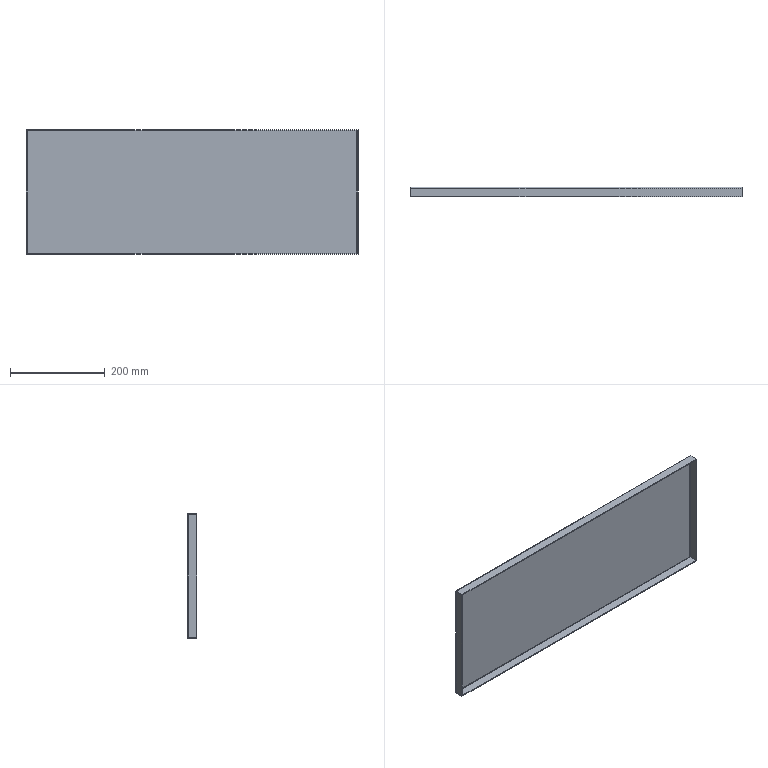Part | STEP file | Transformer Cover 1 | 1 solid | 34 faces | box 700 x 20 x 263 mm | volume 434709 mm3 | plane 26 | cylinder 8 | commonest cylinder face diameters 1 x4 5 x4
STEP:
#1=CARTESIAN_POINT('',(697.5,13.794,89.529));
#2=VERTEX_POINT('',#1);
#3=CARTESIAN_POINT('',(2.5,13.794,89.529));
#4=VERTEX_POINT('',#3);
#5=CARTESIAN_POINT('',(700.,13.794,89.529));
#6=DIRECTION('',(-1.,0.,0.));
#7=VECTOR('',#6,1000.);
#8=LINE('',#5,#7);
#9=EDGE_CURVE('',#2,#4,#8,.T.);
#10=ORIENTED_EDGE('',*,*,#9,.F.);
#11=CARTESIAN_POINT('',(697.5,13.794,-168.471));
#12=VERTEX_POINT('',#11);
#13=CARTESIAN_POINT('',(697.5,13.794,-170.971));
#14=DIRECTION('',(0.,0.,1.));
#15=VECTOR('',#14,1000.);
#16=LINE('',#13,#15);
#17=EDGE_CURVE('',#12,#2,#16,.T.);
#18=ORIENTED_EDGE('',*,*,#17,.F.);
#19=CARTESIAN_POINT('',(2.5,13.794,-168.471));
#20=VERTEX_POINT('',#19);
#21=CARTESIAN_POINT('',(700.,13.794,-168.471));
#22=DIRECTION('',(1.,0.,0.));
#23=VECTOR('',#22,1000.);
#24=LINE('',#21,#23);
#25=EDGE_CURVE('',#20,#12,#24,.T.);
#26=ORIENTED_EDGE('',*,*,#25,.F.);
#27=CARTESIAN_POINT('',(2.5,13.794,-170.971));
#28=DIRECTION('',(0.,0.,-1.));
#29=VECTOR('',#28,1000.);
#30=LINE('',#27,#29);
#31=EDGE_CURVE('',#4,#20,#30,.T.);
#32=ORIENTED_EDGE('',*,*,#31,.F.);
#33=EDGE_LOOP('',(#10,#18,#26,#32));
#34=FACE_OUTER_BOUND('',#33,.T.);
#35=CARTESIAN_POINT('',(700.,13.794,-170.971));
#36=DIRECTION('',(0.,-1.,0.));
#37=DIRECTION('',(0.,0.,-1.));
#38=AXIS2_PLACEMENT_3D('',#35,#36,#37);
#39=PLANE('',#38);
#40=ADVANCED_FACE('',(#34),#39,.F.);
#41=CARTESIAN_POINT('',(0.05051,11.794,89.529));
#42=VERTEX_POINT('',#41);
#43=CARTESIAN_POINT('',(0.,11.294,89.529));
#44=VERTEX_POINT('',#43);
#45=CARTESIAN_POINT('',(2.5,11.294,89.529));
#46=DIRECTION('',(0.,0.,1.));
#47=DIRECTION('',(-1.,0.,0.));
#48=AXIS2_PLACEMENT_3D('',#45,#46,#47);
#49=CIRCLE('',#48,2.5);
#50=EDGE_CURVE('',#42,#44,#49,.T.);
#51=ORIENTED_EDGE('',*,*,#50,.F.);
#52=CARTESIAN_POINT('',(2.5,11.294,89.529));
#53=DIRECTION('',(0.,0.,-1.));
#54=DIRECTION('',(-1.,0.,0.));
#55=AXIS2_PLACEMENT_3D('',#52,#53,#54);
#56=CIRCLE('',#55,2.5);
#57=EDGE_CURVE('',#42,#4,#56,.T.);
#58=ORIENTED_EDGE('',*,*,#57,.T.);
#59=ORIENTED_EDGE('',*,*,#31,.T.);
#60=CARTESIAN_POINT('',(0.05051,11.794,-168.471));
#61=VERTEX_POINT('',#60);
#62=CARTESIAN_POINT('',(2.5,11.294,-168.471));
#63=DIRECTION('',(0.,0.,1.));
#64=DIRECTION('',(-1.,0.,0.));
#65=AXIS2_PLACEMENT_3D('',#62,#63,#64);
#66=CIRCLE('',#65,2.5);
#67=EDGE_CURVE('',#20,#61,#66,.T.);
#68=ORIENTED_EDGE('',*,*,#67,.T.);
#69=CARTESIAN_POINT('',(0.,11.294,-168.471));
#70=VERTEX_POINT('',#69);
#71=CARTESIAN_POINT('',(2.5,11.294,-168.471));
#72=DIRECTION('',(0.,0.,1.));
#73=DIRECTION('',(-1.,0.,0.));
#74=AXIS2_PLACEMENT_3D('',#71,#72,#73);
#75=CIRCLE('',#74,2.5);
#76=EDGE_CURVE('',#61,#70,#75,.T.);
#77=ORIENTED_EDGE('',*,*,#76,.T.);
#78=CARTESIAN_POINT('',(0.,11.294,-168.471));
#79=DIRECTION('',(0.,0.,1.));
#80=VECTOR('',#79,1000.);
#81=LINE('',#78,#80);
#82=EDGE_CURVE('',#70,#44,#81,.T.);
#83=ORIENTED_EDGE('',*,*,#82,.T.);
#84=EDGE_LOOP('',(#51,#58,#59,#68,#77,#83));
#85=FACE_OUTER_BOUND('',#84,.T.);
#86=CARTESIAN_POINT('',(2.5,11.294,-168.471));
#87=DIRECTION('',(0.,0.,-1.));
#88=DIRECTION('',(-1.,0.,0.));
#89=AXIS2_PLACEMENT_3D('',#86,#87,#88);
#90=CYLINDRICAL_SURFACE('',#89,2.5);
#91=ADVANCED_FACE('',(#85),#90,.T.);
#92=ORIENTED_EDGE('',*,*,#9,.T.);
#93=CARTESIAN_POINT('',(0.,13.794,89.529));
#94=VERTEX_POINT('',#93);
#95=CARTESIAN_POINT('',(700.,13.794,89.529));
#96=DIRECTION('',(-1.,0.,0.));
#97=VECTOR('',#96,1000.);
#98=LINE('',#95,#97);
#99=EDGE_CURVE('',#4,#94,#98,.T.);
#100=ORIENTED_EDGE('',*,*,#99,.T.);
#101=CARTESIAN_POINT('',(0.,11.294,92.029));
#102=VERTEX_POINT('',#101);
#103=CARTESIAN_POINT('',(0.,11.294,89.529));
#104=DIRECTION('',(1.,0.,0.));
#105=DIRECTION('',(0.,0.,1.));
#106=AXIS2_PLACEMENT_3D('',#103,#104,#105);
#107=CIRCLE('',#106,2.5);
#108=EDGE_CURVE('',#94,#102,#107,.T.);
#109=ORIENTED_EDGE('',*,*,#108,.T.);
#110=CARTESIAN_POINT('',(700.,11.294,92.029));
#111=VERTEX_POINT('',#110);
#112=CARTESIAN_POINT('',(700.,11.294,92.029));
#113=DIRECTION('',(1.,0.,0.));
#114=VECTOR('',#113,1000.);
#115=LINE('',#112,#114);
#116=EDGE_CURVE('',#102,#111,#115,.T.);
#117=ORIENTED_EDGE('',*,*,#116,.T.);
#118=CARTESIAN_POINT('',(700.,13.794,89.529));
#119=VERTEX_POINT('',#118);
#120=CARTESIAN_POINT('',(700.,11.294,89.529));
#121=DIRECTION('',(-1.,0.,0.));
#122=DIRECTION('',(0.,0.,1.));
#123=AXIS2_PLACEMENT_3D('',#120,#121,#122);
#124=CIRCLE('',#123,2.5);
#125=EDGE_CURVE('',#111,#119,#124,.T.);
#126=ORIENTED_EDGE('',*,*,#125,.T.);
#127=CARTESIAN_POINT('',(700.,13.794,89.529));
#128=DIRECTION('',(-1.,0.,0.));
#129=VECTOR('',#128,1000.);
#130=LINE('',#127,#129);
#131=EDGE_CURVE('',#119,#2,#130,.T.);
#132=ORIENTED_EDGE('',*,*,#131,.T.);
#133=EDGE_LOOP('',(#92,#100,#109,#117,#126,#132));
#134=FACE_OUTER_BOUND('',#133,.T.);
#135=CARTESIAN_POINT('',(700.,11.294,89.529));
#136=DIRECTION('',(-1.,0.,0.));
#137=DIRECTION('',(0.,0.,1.));
#138=AXIS2_PLACEMENT_3D('',#135,#136,#137);
#139=CYLINDRICAL_SURFACE('',#138,2.5);
#140=ADVANCED_FACE('',(#134),#139,.T.);
#141=CARTESIAN_POINT('',(699.949,11.794,-168.471));
#142=VERTEX_POINT('',#141);
#143=CARTESIAN_POINT('',(700.,11.294,-168.471));
#144=VERTEX_POINT('',#143);
#145=CARTESIAN_POINT('',(697.5,11.294,-168.471));
#146=DIRECTION('',(0.,0.,-1.));
#147=DIRECTION('',(1.,0.,0.));
#148=AXIS2_PLACEMENT_3D('',#145,#146,#147);
#149=CIRCLE('',#148,2.5);
#150=EDGE_CURVE('',#142,#144,#149,.T.);
#151=ORIENTED_EDGE('',*,*,#150,.F.);
#152=CARTESIAN_POINT('',(697.5,11.294,-168.471));
#153=DIRECTION('',(0.,0.,1.));
#154=DIRECTION('',(1.,0.,0.));
#155=AXIS2_PLACEMENT_3D('',#152,#153,#154);
#156=CIRCLE('',#155,2.5);
#157=EDGE_CURVE('',#142,#12,#156,.T.);
#158=ORIENTED_EDGE('',*,*,#157,.T.);
#159=ORIENTED_EDGE('',*,*,#17,.T.);
#160=CARTESIAN_POINT('',(699.949,11.794,89.529));
#161=VERTEX_POINT('',#160);
#162=CARTESIAN_POINT('',(697.5,11.294,89.529));
#163=DIRECTION('',(0.,0.,-1.));
#164=DIRECTION('',(1.,0.,0.));
#165=AXIS2_PLACEMENT_3D('',#162,#163,#164);
#166=CIRCLE('',#165,2.5);
#167=EDGE_CURVE('',#2,#161,#166,.T.);
#168=ORIENTED_EDGE('',*,*,#167,.T.);
#169=CARTESIAN_POINT('',(700.,11.294,89.529));
#170=VERTEX_POINT('',#169);
#171=CARTESIAN_POINT('',(697.5,11.294,89.529));
#172=DIRECTION('',(0.,0.,-1.));
#173=DIRECTION('',(1.,0.,0.));
#174=AXIS2_PLACEMENT_3D('',#171,#172,#173);
#175=CIRCLE('',#174,2.5);
#176=EDGE_CURVE('',#161,#170,#175,.T.);
#177=ORIENTED_EDGE('',*,*,#176,.T.);
#178=CARTESIAN_POINT('',(700.,11.294,89.529));
#179=DIRECTION('',(0.,0.,-1.));
#180=VECTOR('',#179,1000.);
#181=LINE('',#178,#180);
#182=EDGE_CURVE('',#170,#144,#181,.T.);
#183=ORIENTED_EDGE('',*,*,#182,.T.);
#184=EDGE_LOOP('',(#151,#158,#159,#168,#177,#183));
#185=FACE_OUTER_BOUND('',#184,.T.);
#186=CARTESIAN_POINT('',(697.5,11.294,89.529));
#187=DIRECTION('',(0.,0.,1.));
#188=DIRECTION('',(1.,0.,0.));
#189=AXIS2_PLACEMENT_3D('',#186,#187,#188);
#190=CYLINDRICAL_SURFACE('',#189,2.5);
#191=ADVANCED_FACE('',(#185),#190,.T.);
#192=CARTESIAN_POINT('',(700.,13.794,-168.471));
#193=VERTEX_POINT('',#192);
#194=CARTESIAN_POINT('',(700.,11.294,-170.971));
#195=VERTEX_POINT('',#194);
#196=CARTESIAN_POINT('',(700.,11.294,-168.471));
#197=DIRECTION('',(-1.,0.,0.));
#198=DIRECTION('',(0.,0.,1.));
#199=AXIS2_PLACEMENT_3D('',#196,#197,#198);
#200=CIRCLE('',#199,2.5);
#201=EDGE_CURVE('',#193,#195,#200,.T.);
#202=ORIENTED_EDGE('',*,*,#201,.T.);
#203=CARTESIAN_POINT('',(0.,11.294,-170.971));
#204=VERTEX_POINT('',#203);
#205=CARTESIAN_POINT('',(700.,11.294,-170.971));
#206=DIRECTION('',(-1.,0.,0.));
#207=VECTOR('',#206,1000.);
#208=LINE('',#205,#207);
#209=EDGE_CURVE('',#195,#204,#208,.T.);
#210=ORIENTED_EDGE('',*,*,#209,.T.);
#211=CARTESIAN_POINT('',(0.,13.794,-168.471));
#212=VERTEX_POINT('',#211);
#213=CARTESIAN_POINT('',(0.,11.294,-168.471));
#214=DIRECTION('',(1.,0.,0.));
#215=DIRECTION('',(0.,0.,1.));
#216=AXIS2_PLACEMENT_3D('',#213,#214,#215);
#217=CIRCLE('',#216,2.5);
#218=EDGE_CURVE('',#204,#212,#217,.T.);
#219=ORIENTED_EDGE('',*,*,#218,.T.);
#220=CARTESIAN_POINT('',(700.,13.794,-168.471));
#221=DIRECTION('',(1.,0.,0.));
#222=VECTOR('',#221,1000.);
#223=LINE('',#220,#222);
#224=EDGE_CURVE('',#212,#20,#223,.T.);
#225=ORIENTED_EDGE('',*,*,#224,.T.);
#226=ORIENTED_EDGE('',*,*,#25,.T.);
#227=CARTESIAN_POINT('',(700.,13.794,-168.471));
#228=DIRECTION('',(1.,0.,0.));
#229=VECTOR('',#228,1000.);
#230=LINE('',#227,#229);
#231=EDGE_CURVE('',#12,#193,#230,.T.);
#232=ORIENTED_EDGE('',*,*,#231,.T.);
#233=EDGE_LOOP('',(#202,#210,#219,#225,#226,#232));
#234=FACE_OUTER_BOUND('',#233,.T.);
#235=CARTESIAN_POINT('',(700.,11.294,-168.471));
#236=DIRECTION('',(-1.,0.,0.));
#237=DIRECTION('',(0.,0.,1.));
#238=AXIS2_PLACEMENT_3D('',#235,#236,#237);
#239=CYLINDRICAL_SURFACE('',#238,2.5);
#240=ADVANCED_FACE('',(#234),#239,.T.);
#241=CARTESIAN_POINT('',(0.,11.794,89.529));
#242=VERTEX_POINT('',#241);
#243=CARTESIAN_POINT('',(700.,11.794,89.529));
#244=DIRECTION('',(-1.,0.,0.));
#245=VECTOR('',#244,1000.);
#246=LINE('',#243,#245);
#247=EDGE_CURVE('',#42,#242,#246,.T.);
#248=ORIENTED_EDGE('',*,*,#247,.T.);
#249=CARTESIAN_POINT('',(0.,11.794,89.529));
#250=DIRECTION('',(0.,1.,0.));
#251=VECTOR('',#250,1000.);
#252=LINE('',#249,#251);
#253=EDGE_CURVE('',#242,#94,#252,.T.);
#254=ORIENTED_EDGE('',*,*,#253,.T.);
#255=ORIENTED_EDGE('',*,*,#99,.F.);
#256=ORIENTED_EDGE('',*,*,#57,.F.);
#257=EDGE_LOOP('',(#248,#254,#255,#256));
#258=FACE_OUTER_BOUND('',#257,.T.);
#259=CARTESIAN_POINT('',(2.5,11.794,89.529));
#260=DIRECTION('',(0.,0.,-1.));
#261=DIRECTION('',(0.,1.,0.));
#262=AXIS2_PLACEMENT_3D('',#259,#260,#261);
#263=PLANE('',#262);
#264=ADVANCED_FACE('',(#258),#263,.T.);
#265=CARTESIAN_POINT('',(0.,-6.206,-168.471));
#266=VERTEX_POINT('',#265);
#267=CARTESIAN_POINT('',(0.,0.,-168.471));
#268=DIRECTION('',(0.,1.,0.));
#269=VECTOR('',#268,1000.);
#270=LINE('',#267,#269);
#271=EDGE_CURVE('',#266,#70,#270,.T.);
#272=ORIENTED_EDGE('',*,*,#271,.F.);
#273=CARTESIAN_POINT('',(0.,-6.206,89.529));
#274=VERTEX_POINT('',#273);
#275=CARTESIAN_POINT('',(0.,-6.206,0.));
#276=DIRECTION('',(0.,0.,-1.));
#277=VECTOR('',#276,1000.);
#278=LINE('',#275,#277);
#279=EDGE_CURVE('',#274,#266,#278,.T.);
#280=ORIENTED_EDGE('',*,*,#279,.F.);
#281=CARTESIAN_POINT('',(0.,0.,89.529));
#282=DIRECTION('',(0.,-1.,0.));
#283=VECTOR('',#282,1000.);
#284=LINE('',#281,#283);
#285=EDGE_CURVE('',#44,#274,#284,.T.);
#286=ORIENTED_EDGE('',*,*,#285,.F.);
#287=ORIENTED_EDGE('',*,*,#82,.F.);
#288=EDGE_LOOP('',(#272,#280,#286,#287));
#289=FACE_OUTER_BOUND('',#288,.T.);
#290=CARTESIAN_POINT('',(0.,0.,0.));
#291=DIRECTION('',(1.,0.,0.));
#292=DIRECTION('',(0.,1.,0.));
#293=AXIS2_PLACEMENT_3D('',#290,#291,#292);
#294=PLANE('',#293);
#295=ADVANCED_FACE('',(#289),#294,.F.);
#296=ORIENTED_EDGE('',*,*,#224,.F.);
#297=CARTESIAN_POINT('',(0.,11.794,-168.471));
#298=VERTEX_POINT('',#297);
#299=CARTESIAN_POINT('',(0.,11.794,-168.471));
#300=DIRECTION('',(0.,-1.,0.));
#301=VECTOR('',#300,1000.);
#302=LINE('',#299,#301);
#303=EDGE_CURVE('',#212,#298,#302,.T.);
#304=ORIENTED_EDGE('',*,*,#303,.T.);
#305=CARTESIAN_POINT('',(700.,11.794,-168.471));
#306=DIRECTION('',(1.,0.,0.));
#307=VECTOR('',#306,1000.);
#308=LINE('',#305,#307);
#309=EDGE_CURVE('',#298,#61,#308,.T.);
#310=ORIENTED_EDGE('',*,*,#309,.T.);
#311=ORIENTED_EDGE('',*,*,#67,.F.);
#312=EDGE_LOOP('',(#296,#304,#310,#311));
#313=FACE_OUTER_BOUND('',#312,.T.);
#314=CARTESIAN_POINT('',(0.,11.794,-168.471));
#315=DIRECTION('',(0.,0.,1.));
#316=DIRECTION('',(0.,-1.,0.));
#317=AXIS2_PLACEMENT_3D('',#314,#315,#316);
#318=PLANE('',#317);
#319=ADVANCED_FACE('',(#313),#318,.T.);
#320=ORIENTED_EDGE('',*,*,#131,.F.);
#321=CARTESIAN_POINT('',(700.,11.794,89.529));
#322=VERTEX_POINT('',#321);
#323=CARTESIAN_POINT('',(700.,11.794,89.529));
#324=DIRECTION('',(0.,-1.,0.));
#325=VECTOR('',#324,1000.);
#326=LINE('',#323,#325);
#327=EDGE_CURVE('',#119,#322,#326,.T.);
#328=ORIENTED_EDGE('',*,*,#327,.T.);
#329=CARTESIAN_POINT('',(700.,11.794,89.529));
#330=DIRECTION('',(-1.,0.,0.));
#331=VECTOR('',#330,1000.);
#332=LINE('',#329,#331);
#333=EDGE_CURVE('',#322,#161,#332,.T.);
#334=ORIENTED_EDGE('',*,*,#333,.T.);
#335=ORIENTED_EDGE('',*,*,#167,.F.);
#336=EDGE_LOOP('',(#320,#328,#334,#335));
#337=FACE_OUTER_BOUND('',#336,.T.);
#338=CARTESIAN_POINT('',(700.,11.794,89.529));
#339=DIRECTION('',(0.,0.,-1.));
#340=DIRECTION('',(0.,1.,0.));
#341=AXIS2_PLACEMENT_3D('',#338,#339,#340);
#342=PLANE('',#341);
#343=ADVANCED_FACE('',(#337),#342,.T.);
#344=ORIENTED_EDGE('',*,*,#125,.F.);
#345=CARTESIAN_POINT('',(700.,-6.206,92.029));
#346=VERTEX_POINT('',#345);
#347=CARTESIAN_POINT('',(700.,13.794,92.029));
#348=DIRECTION('',(0.,-1.,0.));
#349=VECTOR('',#348,1000.);
#350=LINE('',#347,#349);
#351=EDGE_CURVE('',#111,#346,#350,.T.);
#352=ORIENTED_EDGE('',*,*,#351,.T.);
#353=CARTESIAN_POINT('',(700.,-6.206,90.029));
#354=VERTEX_POINT('',#353);
#355=CARTESIAN_POINT('',(700.,-6.206,89.529));
#356=DIRECTION('',(0.,0.,-1.));
#357=VECTOR('',#356,1000.);
#358=LINE('',#355,#357);
#359=EDGE_CURVE('',#346,#354,#358,.T.);
#360=ORIENTED_EDGE('',*,*,#359,.T.);
#361=CARTESIAN_POINT('',(700.,11.294,90.029));
#362=VERTEX_POINT('',#361);
#363=CARTESIAN_POINT('',(700.,11.294,90.029));
#364=DIRECTION('',(0.,1.,0.));
#365=VECTOR('',#364,1000.);
#366=LINE('',#363,#365);
#367=EDGE_CURVE('',#354,#362,#366,.T.);
#368=ORIENTED_EDGE('',*,*,#367,.T.);
#369=CARTESIAN_POINT('',(700.,11.294,89.529));
#370=DIRECTION('',(-1.,0.,0.));
#371=DIRECTION('',(0.,0.,1.));
#372=AXIS2_PLACEMENT_3D('',#369,#370,#371);
#373=CIRCLE('',#372,0.5);
#374=EDGE_CURVE('',#362,#322,#373,.T.);
#375=ORIENTED_EDGE('',*,*,#374,.T.);
#376=ORIENTED_EDGE('',*,*,#327,.F.);
#377=EDGE_LOOP('',(#344,#352,#360,#368,#375,#376));
#378=FACE_OUTER_BOUND('',#377,.T.);
#379=CARTESIAN_POINT('',(700.,13.794,89.529));
#380=DIRECTION('',(1.,0.,0.));
#381=DIRECTION('',(0.,0.,-1.));
#382=AXIS2_PLACEMENT_3D('',#379,#380,#381);
#383=PLANE('',#382);
#384=ADVANCED_FACE('',(#378),#383,.T.);
#385=CARTESIAN_POINT('',(0.,-6.206,92.029));
#386=VERTEX_POINT('',#385);
#387=CARTESIAN_POINT('',(700.,-6.206,92.029));
#388=DIRECTION('',(-1.,0.,0.));
#389=VECTOR('',#388,1000.);
#390=LINE('',#387,#389);
#391=EDGE_CURVE('',#346,#386,#390,.T.);
#392=ORIENTED_EDGE('',*,*,#391,.F.);
#393=ORIENTED_EDGE('',*,*,#351,.F.);
#394=ORIENTED_EDGE('',*,*,#116,.F.);
#395=CARTESIAN_POINT('',(0.,13.794,92.029));
#396=DIRECTION('',(0.,1.,0.));
#397=VECTOR('',#396,1000.);
#398=LINE('',#395,#397);
#399=EDGE_CURVE('',#386,#102,#398,.T.);
#400=ORIENTED_EDGE('',*,*,#399,.F.);
#401=EDGE_LOOP('',(#392,#393,#394,#400));
#402=FACE_OUTER_BOUND('',#401,.T.);
#403=CARTESIAN_POINT('',(700.,13.794,92.029));
#404=DIRECTION('',(0.,0.,-1.));
#405=DIRECTION('',(-1.,0.,0.));
#406=AXIS2_PLACEMENT_3D('',#403,#404,#405);
#407=PLANE('',#406);
#408=ADVANCED_FACE('',(#402),#407,.F.);
#409=ORIENTED_EDGE('',*,*,#253,.F.);
#410=CARTESIAN_POINT('',(0.,11.294,90.029));
#411=VERTEX_POINT('',#410);
#412=CARTESIAN_POINT('',(0.,11.294,89.529));
#413=DIRECTION('',(1.,0.,0.));
#414=DIRECTION('',(0.,0.,1.));
#415=AXIS2_PLACEMENT_3D('',#412,#413,#414);
#416=CIRCLE('',#415,0.5);
#417=EDGE_CURVE('',#242,#411,#416,.T.);
#418=ORIENTED_EDGE('',*,*,#417,.T.);
#419=CARTESIAN_POINT('',(0.,-6.206,90.029));
#420=VERTEX_POINT('',#419);
#421=CARTESIAN_POINT('',(0.,11.794,90.029));
#422=DIRECTION('',(0.,-1.,0.));
#423=VECTOR('',#422,1000.);
#424=LINE('',#421,#423);
#425=EDGE_CURVE('',#411,#420,#424,.T.);
#426=ORIENTED_EDGE('',*,*,#425,.T.);
#427=CARTESIAN_POINT('',(0.,-6.206,89.529));
#428=DIRECTION('',(0.,0.,1.));
#429=VECTOR('',#428,1000.);
#430=LINE('',#427,#429);
#431=EDGE_CURVE('',#420,#386,#430,.T.);
#432=ORIENTED_EDGE('',*,*,#431,.T.);
#433=ORIENTED_EDGE('',*,*,#399,.T.);
#434=ORIENTED_EDGE('',*,*,#108,.F.);
#435=EDGE_LOOP('',(#409,#418,#426,#432,#433,#434));
#436=FACE_OUTER_BOUND('',#435,.T.);
#437=CARTESIAN_POINT('',(0.,11.294,92.029));
#438=DIRECTION('',(-1.,0.,0.));
#439=DIRECTION('',(0.,0.,1.));
#440=AXIS2_PLACEMENT_3D('',#437,#438,#439);
#441=PLANE('',#440);
#442=ADVANCED_FACE('',(#436),#441,.T.);
#443=CARTESIAN_POINT('',(700.,11.794,-168.471));
#444=VERTEX_POINT('',#443);
#445=CARTESIAN_POINT('',(700.,11.794,-168.471));
#446=DIRECTION('',(1.,0.,0.));
#447=VECTOR('',#446,1000.);
#448=LINE('',#445,#447);
#449=EDGE_CURVE('',#142,#444,#448,.T.);
#450=ORIENTED_EDGE('',*,*,#449,.T.);
#451=CARTESIAN_POINT('',(700.,11.794,-168.471));
#452=DIRECTION('',(0.,1.,0.));
#453=VECTOR('',#452,1000.);
#454=LINE('',#451,#453);
#455=EDGE_CURVE('',#444,#193,#454,.T.);
#456=ORIENTED_EDGE('',*,*,#455,.T.);
#457=ORIENTED_EDGE('',*,*,#231,.F.);
#458=ORIENTED_EDGE('',*,*,#157,.F.);
#459=EDGE_LOOP('',(#450,#456,#457,#458));
#460=FACE_OUTER_BOUND('',#459,.T.);
#461=CARTESIAN_POINT('',(697.5,11.794,-168.471));
#462=DIRECTION('',(0.,0.,1.));
#463=DIRECTION('',(0.,-1.,0.));
#464=AXIS2_PLACEMENT_3D('',#461,#462,#463);
#465=PLANE('',#464);
#466=ADVANCED_FACE('',(#460),#465,.T.);
#467=CARTESIAN_POINT('',(700.,-6.206,89.529));
#468=VERTEX_POINT('',#467);
#469=CARTESIAN_POINT('',(700.,0.,89.529));
#470=DIRECTION('',(0.,-1.,0.));
#471=VECTOR('',#470,1000.);
#472=LINE('',#469,#471);
#473=EDGE_CURVE('',#170,#468,#472,.T.);
#474=ORIENTED_EDGE('',*,*,#473,.T.);
#475=CARTESIAN_POINT('',(700.,-6.206,-168.471));
#476=VERTEX_POINT('',#475);
#477=CARTESIAN_POINT('',(700.,-6.206,0.));
#478=DIRECTION('',(0.,0.,-1.));
#479=VECTOR('',#478,1000.);
#480=LINE('',#477,#479);
#481=EDGE_CURVE('',#468,#476,#480,.T.);
#482=ORIENTED_EDGE('',*,*,#481,.T.);
#483=CARTESIAN_POINT('',(700.,0.,-168.471));
#484=DIRECTION('',(0.,1.,0.));
#485=VECTOR('',#484,1000.);
#486=LINE('',#483,#485);
#487=EDGE_CURVE('',#476,#144,#486,.T.);
#488=ORIENTED_EDGE('',*,*,#487,.T.);
#489=ORIENTED_EDGE('',*,*,#182,.F.);
#490=EDGE_LOOP('',(#474,#482,#488,#489));
#491=FACE_OUTER_BOUND('',#490,.T.);
#492=CARTESIAN_POINT('',(700.,0.,0.));
#493=DIRECTION('',(1.,0.,0.));
#494=DIRECTION('',(0.,1.,0.));
#495=AXIS2_PLACEMENT_3D('',#492,#493,#494);
#496=PLANE('',#495);
#497=ADVANCED_FACE('',(#491),#496,.T.);
#498=ORIENTED_EDGE('',*,*,#209,.F.);
#499=CARTESIAN_POINT('',(700.,-6.206,-170.971));
#500=VERTEX_POINT('',#499);
#501=CARTESIAN_POINT('',(700.,13.794,-170.971));
#502=DIRECTION('',(0.,1.,0.));
#503=VECTOR('',#502,1000.);
#504=LINE('',#501,#503);
#505=EDGE_CURVE('',#500,#195,#504,.T.);
#506=ORIENTED_EDGE('',*,*,#505,.F.);
#507=CARTESIAN_POINT('',(0.,-6.206,-170.971));
#508=VERTEX_POINT('',#507);
#509=CARTESIAN_POINT('',(700.,-6.206,-170.971));
#510=DIRECTION('',(1.,0.,0.));
#511=VECTOR('',#510,1000.);
#512=LINE('',#509,#511);
#513=EDGE_CURVE('',#508,#500,#512,.T.);
#514=ORIENTED_EDGE('',*,*,#513,.F.);
#515=CARTESIAN_POINT('',(0.,13.794,-170.971));
#516=DIRECTION('',(0.,-1.,0.));
#517=VECTOR('',#516,1000.);
#518=LINE('',#515,#517);
#519=EDGE_CURVE('',#204,#508,#518,.T.);
#520=ORIENTED_EDGE('',*,*,#519,.F.);
#521=EDGE_LOOP('',(#498,#506,#514,#520));
#522=FACE_OUTER_BOUND('',#521,.T.);
#523=CARTESIAN_POINT('',(700.,13.794,-170.971));
#524=DIRECTION('',(0.,0.,1.));
#525=DIRECTION('',(1.,0.,0.));
#526=AXIS2_PLACEMENT_3D('',#523,#524,#525);
#527=PLANE('',#526);
#528=ADVANCED_FACE('',(#522),#527,.F.);
#529=ORIENTED_EDGE('',*,*,#455,.F.);
#530=CARTESIAN_POINT('',(700.,11.294,-168.971));
#531=VERTEX_POINT('',#530);
#532=CARTESIAN_POINT('',(700.,11.294,-168.471));
#533=DIRECTION('',(-1.,0.,0.));
#534=DIRECTION('',(0.,0.,1.));
#535=AXIS2_PLACEMENT_3D('',#532,#533,#534);
#536=CIRCLE('',#535,0.5);
#537=EDGE_CURVE('',#444,#531,#536,.T.);
#538=ORIENTED_EDGE('',*,*,#537,.T.);
#539=CARTESIAN_POINT('',(700.,-6.206,-168.971));
#540=VERTEX_POINT('',#539);
#541=CARTESIAN_POINT('',(700.,11.794,-168.971));
#542=DIRECTION('',(0.,-1.,0.));
#543=VECTOR('',#542,1000.);
#544=LINE('',#541,#543);
#545=EDGE_CURVE('',#531,#540,#544,.T.);
#546=ORIENTED_EDGE('',*,*,#545,.T.);
#547=CARTESIAN_POINT('',(700.,-6.206,-168.471));
#548=DIRECTION('',(0.,0.,-1.));
#549=VECTOR('',#548,1000.);
#550=LINE('',#547,#549);
#551=EDGE_CURVE('',#540,#500,#550,.T.);
#552=ORIENTED_EDGE('',*,*,#551,.T.);
#553=ORIENTED_EDGE('',*,*,#505,.T.);
#554=ORIENTED_EDGE('',*,*,#201,.F.);
#555=EDGE_LOOP('',(#529,#538,#546,#552,#553,#554));
#556=FACE_OUTER_BOUND('',#555,.T.);
#557=CARTESIAN_POINT('',(700.,11.294,-170.971));
#558=DIRECTION('',(1.,0.,0.));
#559=DIRECTION('',(0.,0.,-1.));
#560=AXIS2_PLACEMENT_3D('',#557,#558,#559);
#561=PLANE('',#560);
#562=ADVANCED_FACE('',(#556),#561,.T.);
#563=ORIENTED_EDGE('',*,*,#218,.F.);
#564=ORIENTED_EDGE('',*,*,#519,.T.);
#565=CARTESIAN_POINT('',(0.,-6.206,-168.971));
#566=VERTEX_POINT('',#565);
#567=CARTESIAN_POINT('',(0.,-6.206,89.529));
#568=DIRECTION('',(0.,0.,-1.));
#569=VECTOR('',#568,1000.);
#570=LINE('',#567,#569);
#571=EDGE_CURVE('',#566,#508,#570,.T.);
#572=ORIENTED_EDGE('',*,*,#571,.F.);
#573=CARTESIAN_POINT('',(0.,11.294,-168.971));
#574=VERTEX_POINT('',#573);
#575=CARTESIAN_POINT('',(0.,11.294,-168.971));
#576=DIRECTION('',(0.,-1.,0.));
#577=VECTOR('',#576,1000.);
#578=LINE('',#575,#577);
#579=EDGE_CURVE('',#574,#566,#578,.T.);
#580=ORIENTED_EDGE('',*,*,#579,.F.);
#581=CARTESIAN_POINT('',(0.,11.294,-168.471));
#582=DIRECTION('',(1.,0.,0.));
#583=DIRECTION('',(0.,0.,1.));
#584=AXIS2_PLACEMENT_3D('',#581,#582,#583);
#585=CIRCLE('',#584,0.5);
#586=EDGE_CURVE('',#574,#298,#585,.T.);
#587=ORIENTED_EDGE('',*,*,#586,.T.);
#588=ORIENTED_EDGE('',*,*,#303,.F.);
#589=EDGE_LOOP('',(#563,#564,#572,#580,#587,#588));
#590=FACE_OUTER_BOUND('',#589,.T.);
#591=CARTESIAN_POINT('',(0.,13.794,-168.471));
#592=DIRECTION('',(-1.,0.,0.));
#593=DIRECTION('',(0.,0.,1.));
#594=AXIS2_PLACEMENT_3D('',#591,#592,#593);
#595=PLANE('',#594);
#596=ADVANCED_FACE('',(#590),#595,.T.);
#597=CARTESIAN_POINT('',(2.,11.294,-168.471));
#598=VERTEX_POINT('',#597);
#599=CARTESIAN_POINT('',(2.,-6.206,-168.471));
#600=VERTEX_POINT('',#599);
#601=CARTESIAN_POINT('',(2.,-6.206,-168.471));
#602=DIRECTION('',(0.,-1.,0.));
#603=VECTOR('',#602,1000.);
#604=LINE('',#601,#603);
#605=EDGE_CURVE('',#598,#600,#604,.T.);
#606=ORIENTED_EDGE('',*,*,#605,.T.);
#607=CARTESIAN_POINT('',(0.,-6.206,-168.471));
#608=DIRECTION('',(-1.,0.,0.));
#609=VECTOR('',#608,1000.);
#610=LINE('',#607,#609);
#611=EDGE_CURVE('',#600,#266,#610,.T.);
#612=ORIENTED_EDGE('',*,*,#611,.T.);
#613=ORIENTED_EDGE('',*,*,#271,.T.);
#614=ORIENTED_EDGE('',*,*,#76,.F.);
#615=CARTESIAN_POINT('',(2.5,11.794,-168.471));
#616=VERTEX_POINT('',#615);
#617=CARTESIAN_POINT('',(2.5,11.794,-168.471));
#618=DIRECTION('',(-1.,0.,0.));
#619=VECTOR('',#618,1000.);
#620=LINE('',#617,#619);
#621=EDGE_CURVE('',#616,#61,#620,.T.);
#622=ORIENTED_EDGE('',*,*,#621,.F.);
#623=CARTESIAN_POINT('',(2.5,11.294,-168.471));
#624=DIRECTION('',(0.,0.,-1.));
#625=DIRECTION('',(-1.,0.,0.));
#626=AXIS2_PLACEMENT_3D('',#623,#624,#625);
#627=CIRCLE('',#626,0.5);
#628=EDGE_CURVE('',#598,#616,#627,.T.);
#629=ORIENTED_EDGE('',*,*,#628,.F.);
#630=EDGE_LOOP('',(#606,#612,#613,#614,#622,#629));
#631=FACE_OUTER_BOUND('',#630,.T.);
#632=CARTESIAN_POINT('',(0.,-6.206,-168.471));
#633=DIRECTION('',(0.,0.,-1.));
#634=DIRECTION('',(-1.,0.,0.));
#635=AXIS2_PLACEMENT_3D('',#632,#633,#634);
#636=PLANE('',#635);
#637=ADVANCED_FACE('',(#631),#636,.T.);
#638=ORIENTED_EDGE('',*,*,#279,.T.);
#639=ORIENTED_EDGE('',*,*,#611,.F.);
#640=CARTESIAN_POINT('',(2.,-6.206,89.529));
#641=VERTEX_POINT('',#640);
#642=CARTESIAN_POINT('',(2.,-6.206,89.529));
#643=DIRECTION('',(0.,0.,1.));
#644=VECTOR('',#643,1000.);
#645=LINE('',#642,#644);
#646=EDGE_CURVE('',#600,#641,#645,.T.);
#647=ORIENTED_EDGE('',*,*,#646,.T.);
#648=CARTESIAN_POINT('',(0.,-6.206,89.529));
#649=DIRECTION('',(-1.,0.,0.));
#650=VECTOR('',#649,1000.);
#651=LINE('',#648,#650);
#652=EDGE_CURVE('',#641,#274,#651,.T.);
#653=ORIENTED_EDGE('',*,*,#652,.T.);
#654=EDGE_LOOP('',(#638,#639,#647,#653));
#655=FACE_OUTER_BOUND('',#654,.T.);
#656=CARTESIAN_POINT('',(0.,-6.206,89.529));
#657=DIRECTION('',(0.,-1.,0.));
#658=DIRECTION('',(1.,0.,0.));
#659=AXIS2_PLACEMENT_3D('',#656,#657,#658);
#660=PLANE('',#659);
#661=ADVANCED_FACE('',(#655),#660,.T.);
#662=ORIENTED_EDGE('',*,*,#285,.T.);
#663=ORIENTED_EDGE('',*,*,#652,.F.);
#664=CARTESIAN_POINT('',(2.,11.294,89.529));
#665=VERTEX_POINT('',#664);
#666=CARTESIAN_POINT('',(2.,11.794,89.529));
#667=DIRECTION('',(0.,1.,0.));
#668=VECTOR('',#667,1000.);
#669=LINE('',#666,#668);
#670=EDGE_CURVE('',#641,#665,#669,.T.);
#671=ORIENTED_EDGE('',*,*,#670,.T.);
#672=CARTESIAN_POINT('',(2.5,11.794,89.529));
#673=VERTEX_POINT('',#672);
#674=CARTESIAN_POINT('',(2.5,11.294,89.529));
#675=DIRECTION('',(0.,0.,-1.));
#676=DIRECTION('',(-1.,0.,0.));
#677=AXIS2_PLACEMENT_3D('',#674,#675,#676);
#678=CIRCLE('',#677,0.5);
#679=EDGE_CURVE('',#665,#673,#678,.T.);
#680=ORIENTED_EDGE('',*,*,#679,.T.);
#681=CARTESIAN_POINT('',(2.5,11.794,89.529));
#682=DIRECTION('',(-1.,0.,0.));
#683=VECTOR('',#682,1000.);
#684=LINE('',#681,#683);
#685=EDGE_CURVE('',#673,#42,#684,.T.);
#686=ORIENTED_EDGE('',*,*,#685,.T.);
#687=ORIENTED_EDGE('',*,*,#50,.T.);
#688=EDGE_LOOP('',(#662,#663,#671,#680,#686,#687));
#689=FACE_OUTER_BOUND('',#688,.T.);
#690=CARTESIAN_POINT('',(0.,11.794,89.529));
#691=DIRECTION('',(0.,0.,1.));
#692=DIRECTION('',(0.,-1.,0.));
#693=AXIS2_PLACEMENT_3D('',#690,#691,#692);
#694=PLANE('',#693);
#695=ADVANCED_FACE('',(#689),#694,.T.);
#696=ORIENTED_EDGE('',*,*,#359,.F.);
#697=ORIENTED_EDGE('',*,*,#391,.T.);
#698=ORIENTED_EDGE('',*,*,#431,.F.);
#699=CARTESIAN_POINT('',(700.,-6.206,90.029));
#700=DIRECTION('',(1.,0.,0.));
#701=VECTOR('',#700,1000.);
#702=LINE('',#699,#701);
#703=EDGE_CURVE('',#420,#354,#702,.T.);
#704=ORIENTED_EDGE('',*,*,#703,.T.);
#705=EDGE_LOOP('',(#696,#697,#698,#704));
#706=FACE_OUTER_BOUND('',#705,.T.);
#707=CARTESIAN_POINT('',(700.,-6.206,90.029));
#708=DIRECTION('',(0.,-1.,0.));
#709=DIRECTION('',(0.,0.,-1.));
#710=AXIS2_PLACEMENT_3D('',#707,#708,#709);
#711=PLANE('',#710);
#712=ADVANCED_FACE('',(#706),#711,.T.);
#713=ORIENTED_EDGE('',*,*,#481,.F.);
#714=CARTESIAN_POINT('',(698.,-6.206,89.529));
#715=VERTEX_POINT('',#714);
#716=CARTESIAN_POINT('',(700.,-6.206,89.529));
#717=DIRECTION('',(-1.,0.,0.));
#718=VECTOR('',#717,1000.);
#719=LINE('',#716,#718);
#720=EDGE_CURVE('',#468,#715,#719,.T.);
#721=ORIENTED_EDGE('',*,*,#720,.T.);
#722=CARTESIAN_POINT('',(698.,-6.206,-168.471));
#723=VERTEX_POINT('',#722);
#724=CARTESIAN_POINT('',(698.,-6.206,89.529));
#725=DIRECTION('',(0.,0.,-1.));
#726=VECTOR('',#725,1000.);
#727=LINE('',#724,#726);
#728=EDGE_CURVE('',#715,#723,#727,.T.);
#729=ORIENTED_EDGE('',*,*,#728,.T.);
#730=CARTESIAN_POINT('',(700.,-6.206,-168.471));
#731=DIRECTION('',(1.,0.,0.));
#732=VECTOR('',#731,1000.);
#733=LINE('',#730,#732);
#734=EDGE_CURVE('',#723,#476,#733,.T.);
#735=ORIENTED_EDGE('',*,*,#734,.T.);
#736=EDGE_LOOP('',(#713,#721,#729,#735));
#737=FACE_OUTER_BOUND('',#736,.T.);
#738=CARTESIAN_POINT('',(700.,-6.206,89.529));
#739=DIRECTION('',(0.,-1.,0.));
#740=DIRECTION('',(1.,0.,0.));
#741=AXIS2_PLACEMENT_3D('',#738,#739,#740);
#742=PLANE('',#741);
#743=ADVANCED_FACE('',(#737),#742,.T.);
#744=CARTESIAN_POINT('',(698.,11.294,89.529));
#745=VERTEX_POINT('',#744);
#746=CARTESIAN_POINT('',(698.,11.794,89.529));
#747=DIRECTION('',(0.,-1.,0.));
#748=VECTOR('',#747,1000.);
#749=LINE('',#746,#748);
#750=EDGE_CURVE('',#745,#715,#749,.T.);
#751=ORIENTED_EDGE('',*,*,#750,.T.);
#752=ORIENTED_EDGE('',*,*,#720,.F.);
#753=ORIENTED_EDGE('',*,*,#473,.F.);
#754=ORIENTED_EDGE('',*,*,#176,.F.);
#755=CARTESIAN_POINT('',(697.5,11.794,89.529));
#756=VERTEX_POINT('',#755);
#757=CARTESIAN_POINT('',(697.5,11.794,89.529));
#758=DIRECTION('',(1.,0.,0.));
#759=VECTOR('',#758,1000.);
#760=LINE('',#757,#759);
#761=EDGE_CURVE('',#756,#161,#760,.T.);
#762=ORIENTED_EDGE('',*,*,#761,.F.);
#763=CARTESIAN_POINT('',(697.5,11.294,89.529));
#764=DIRECTION('',(0.,0.,1.));
#765=DIRECTION('',(1.,0.,0.));
#766=AXIS2_PLACEMENT_3D('',#763,#764,#765);
#767=CIRCLE('',#766,0.5);
#768=EDGE_CURVE('',#745,#756,#767,.T.);
#769=ORIENTED_EDGE('',*,*,#768,.F.);
#770=EDGE_LOOP('',(#751,#752,#753,#754,#762,#769));
#771=FACE_OUTER_BOUND('',#770,.T.);
#772=CARTESIAN_POINT('',(700.,11.794,89.529));
#773=DIRECTION('',(0.,0.,1.));
#774=DIRECTION('',(1.,0.,0.));
#775=AXIS2_PLACEMENT_3D('',#772,#773,#774);
#776=PLANE('',#775);
#777=ADVANCED_FACE('',(#771),#776,.T.);
#778=ORIENTED_EDGE('',*,*,#487,.F.);
#779=ORIENTED_EDGE('',*,*,#734,.F.);
#780=CARTESIAN_POINT('',(698.,11.294,-168.471));
#781=VERTEX_POINT('',#780);
#782=CARTESIAN_POINT('',(698.,-6.206,-168.471));
#783=DIRECTION('',(0.,1.,0.));
#784=VECTOR('',#783,1000.);
#785=LINE('',#782,#784);
#786=EDGE_CURVE('',#723,#781,#785,.T.);
#787=ORIENTED_EDGE('',*,*,#786,.T.);
#788=CARTESIAN_POINT('',(697.5,11.794,-168.471));
#789=VERTEX_POINT('',#788);
#790=CARTESIAN_POINT('',(697.5,11.294,-168.471));
#791=DIRECTION('',(0.,0.,1.));
#792=DIRECTION('',(1.,0.,0.));
#793=AXIS2_PLACEMENT_3D('',#790,#791,#792);
#794=CIRCLE('',#793,0.5);
#795=EDGE_CURVE('',#781,#789,#794,.T.);
#796=ORIENTED_EDGE('',*,*,#795,.T.);
#797=CARTESIAN_POINT('',(697.5,11.794,-168.471));
#798=DIRECTION('',(1.,0.,0.));
#799=VECTOR('',#798,1000.);
#800=LINE('',#797,#799);
#801=EDGE_CURVE('',#789,#142,#800,.T.);
#802=ORIENTED_EDGE('',*,*,#801,.T.);
#803=ORIENTED_EDGE('',*,*,#150,.T.);
#804=EDGE_LOOP('',(#778,#779,#787,#796,#802,#803));
#805=FACE_OUTER_BOUND('',#804,.T.);
#806=CARTESIAN_POINT('',(700.,-6.206,-168.471));
#807=DIRECTION('',(0.,0.,-1.));
#808=DIRECTION('',(-1.,0.,0.));
#809=AXIS2_PLACEMENT_3D('',#806,#807,#808);
#810=PLANE('',#809);
#811=ADVANCED_FACE('',(#805),#810,.T.);
#812=ORIENTED_EDGE('',*,*,#551,.F.);
#813=CARTESIAN_POINT('',(700.,-6.206,-168.971));
#814=DIRECTION('',(-1.,0.,0.));
#815=VECTOR('',#814,1000.);
#816=LINE('',#813,#815);
#817=EDGE_CURVE('',#540,#566,#816,.T.);
#818=ORIENTED_EDGE('',*,*,#817,.T.);
#819=ORIENTED_EDGE('',*,*,#571,.T.);
#820=ORIENTED_EDGE('',*,*,#513,.T.);
#821=EDGE_LOOP('',(#812,#818,#819,#820));
#822=FACE_OUTER_BOUND('',#821,.T.);
#823=CARTESIAN_POINT('',(700.,-6.206,-170.971));
#824=DIRECTION('',(0.,-1.,0.));
#825=DIRECTION('',(0.,0.,-1.));
#826=AXIS2_PLACEMENT_3D('',#823,#824,#825);
#827=PLANE('',#826);
#828=ADVANCED_FACE('',(#822),#827,.T.);
#829=ORIENTED_EDGE('',*,*,#670,.F.);
#830=ORIENTED_EDGE('',*,*,#646,.F.);
#831=ORIENTED_EDGE('',*,*,#605,.F.);
#832=CARTESIAN_POINT('',(2.,11.294,0.));
#833=DIRECTION('',(0.,0.,1.));
#834=VECTOR('',#833,1000.);
#835=LINE('',#832,#834);
#836=EDGE_CURVE('',#598,#665,#835,.T.);
#837=ORIENTED_EDGE('',*,*,#836,.T.);
#838=EDGE_LOOP('',(#829,#830,#831,#837));
#839=FACE_OUTER_BOUND('',#838,.T.);
#840=CARTESIAN_POINT('',(2.,0.,0.));
#841=DIRECTION('',(1.,0.,0.));
#842=DIRECTION('',(0.,1.,0.));
#843=AXIS2_PLACEMENT_3D('',#840,#841,#842);
#844=PLANE('',#843);
#845=ADVANCED_FACE('',(#839),#844,.T.);
#846=ORIENTED_EDGE('',*,*,#367,.F.);
#847=ORIENTED_EDGE('',*,*,#703,.F.);
#848=ORIENTED_EDGE('',*,*,#425,.F.);
#849=CARTESIAN_POINT('',(700.,11.294,90.029));
#850=DIRECTION('',(1.,0.,0.));
#851=VECTOR('',#850,1000.);
#852=LINE('',#849,#851);
#853=EDGE_CURVE('',#411,#362,#852,.T.);
#854=ORIENTED_EDGE('',*,*,#853,.T.);
#855=EDGE_LOOP('',(#846,#847,#848,#854));
#856=FACE_OUTER_BOUND('',#855,.T.);
#857=CARTESIAN_POINT('',(700.,13.794,90.029));
#858=DIRECTION('',(0.,0.,-1.));
#859=DIRECTION('',(-1.,0.,0.));
#860=AXIS2_PLACEMENT_3D('',#857,#858,#859);
#861=PLANE('',#860);
#862=ADVANCED_FACE('',(#856),#861,.T.);
#863=ORIENTED_EDGE('',*,*,#786,.F.);
#864=ORIENTED_EDGE('',*,*,#728,.F.);
#865=ORIENTED_EDGE('',*,*,#750,.F.);
#866=CARTESIAN_POINT('',(698.,11.294,0.));
#867=DIRECTION('',(0.,0.,1.));
#868=VECTOR('',#867,1000.);
#869=LINE('',#866,#868);
#870=EDGE_CURVE('',#781,#745,#869,.T.);
#871=ORIENTED_EDGE('',*,*,#870,.F.);
#872=EDGE_LOOP('',(#863,#864,#865,#871));
#873=FACE_OUTER_BOUND('',#872,.T.);
#874=CARTESIAN_POINT('',(698.,0.,0.));
#875=DIRECTION('',(1.,0.,0.));
#876=DIRECTION('',(0.,1.,0.));
#877=AXIS2_PLACEMENT_3D('',#874,#875,#876);
#878=PLANE('',#877);
#879=ADVANCED_FACE('',(#873),#878,.F.);
#880=ORIENTED_EDGE('',*,*,#545,.F.);
#881=CARTESIAN_POINT('',(700.,11.294,-168.971));
#882=DIRECTION('',(-1.,0.,0.));
#883=VECTOR('',#882,1000.);
#884=LINE('',#881,#883);
#885=EDGE_CURVE('',#531,#574,#884,.T.);
#886=ORIENTED_EDGE('',*,*,#885,.T.);
#887=ORIENTED_EDGE('',*,*,#579,.T.);
#888=ORIENTED_EDGE('',*,*,#817,.F.);
#889=EDGE_LOOP('',(#880,#886,#887,#888));
#890=FACE_OUTER_BOUND('',#889,.T.);
#891=CARTESIAN_POINT('',(700.,13.794,-168.971));
#892=DIRECTION('',(0.,0.,1.));
#893=DIRECTION('',(1.,0.,0.));
#894=AXIS2_PLACEMENT_3D('',#891,#892,#893);
#895=PLANE('',#894);
#896=ADVANCED_FACE('',(#890),#895,.T.);
#897=ORIENTED_EDGE('',*,*,#679,.F.);
#898=ORIENTED_EDGE('',*,*,#836,.F.);
#899=ORIENTED_EDGE('',*,*,#628,.T.);
#900=CARTESIAN_POINT('',(2.5,11.794,-168.471));
#901=DIRECTION('',(0.,0.,-1.));
#902=VECTOR('',#901,1000.);
#903=LINE('',#900,#902);
#904=EDGE_CURVE('',#673,#616,#903,.T.);
#905=ORIENTED_EDGE('',*,*,#904,.F.);
#906=EDGE_LOOP('',(#897,#898,#899,#905));
#907=FACE_OUTER_BOUND('',#906,.T.);
#908=CARTESIAN_POINT('',(2.5,11.294,-168.471));
#909=DIRECTION('',(0.,0.,-1.));
#910=DIRECTION('',(-1.,0.,0.));
#911=AXIS2_PLACEMENT_3D('',#908,#909,#910);
#912=CYLINDRICAL_SURFACE('',#911,0.5);
#913=ADVANCED_FACE('',(#907),#912,.F.);
#914=ORIENTED_EDGE('',*,*,#885,.F.);
#915=ORIENTED_EDGE('',*,*,#537,.F.);
#916=ORIENTED_EDGE('',*,*,#449,.F.);
#917=ORIENTED_EDGE('',*,*,#801,.F.);
#918=CARTESIAN_POINT('',(700.,11.794,-168.471));
#919=DIRECTION('',(1.,0.,0.));
#920=VECTOR('',#919,1000.);
#921=LINE('',#918,#920);
#922=EDGE_CURVE('',#616,#789,#921,.T.);
#923=ORIENTED_EDGE('',*,*,#922,.F.);
#924=ORIENTED_EDGE('',*,*,#621,.T.);
#925=ORIENTED_EDGE('',*,*,#309,.F.);
#926=ORIENTED_EDGE('',*,*,#586,.F.);
#927=EDGE_LOOP('',(#914,#915,#916,#917,#923,#924,#925,#926));
#928=FACE_OUTER_BOUND('',#927,.T.);
#929=CARTESIAN_POINT('',(700.,11.294,-168.471));
#930=DIRECTION('',(-1.,0.,0.));
#931=DIRECTION('',(0.,0.,1.));
#932=AXIS2_PLACEMENT_3D('',#929,#930,#931);
#933=CYLINDRICAL_SURFACE('',#932,0.5);
#934=ADVANCED_FACE('',(#928),#933,.F.);
#935=ORIENTED_EDGE('',*,*,#247,.F.);
#936=ORIENTED_EDGE('',*,*,#685,.F.);
#937=CARTESIAN_POINT('',(700.,11.794,89.529));
#938=DIRECTION('',(-1.,0.,0.));
#939=VECTOR('',#938,1000.);
#940=LINE('',#937,#939);
#941=EDGE_CURVE('',#756,#673,#940,.T.);
#942=ORIENTED_EDGE('',*,*,#941,.F.);
#943=ORIENTED_EDGE('',*,*,#761,.T.);
#944=ORIENTED_EDGE('',*,*,#333,.F.);
#945=ORIENTED_EDGE('',*,*,#374,.F.);
#946=ORIENTED_EDGE('',*,*,#853,.F.);
#947=ORIENTED_EDGE('',*,*,#417,.F.);
#948=EDGE_LOOP('',(#935,#936,#942,#943,#944,#945,#946,#947));
#949=FACE_OUTER_BOUND('',#948,.T.);
#950=CARTESIAN_POINT('',(700.,11.294,89.529));
#951=DIRECTION('',(-1.,0.,0.));
#952=DIRECTION('',(0.,0.,1.));
#953=AXIS2_PLACEMENT_3D('',#950,#951,#952);
#954=CYLINDRICAL_SURFACE('',#953,0.5);
#955=ADVANCED_FACE('',(#949),#954,.F.);
#956=ORIENTED_EDGE('',*,*,#795,.F.);
#957=ORIENTED_EDGE('',*,*,#870,.T.);
#958=ORIENTED_EDGE('',*,*,#768,.T.);
#959=CARTESIAN_POINT('',(697.5,11.794,89.529));
#960=DIRECTION('',(0.,0.,1.));
#961=VECTOR('',#960,1000.);
#962=LINE('',#959,#961);
#963=EDGE_CURVE('',#789,#756,#962,.T.);
#964=ORIENTED_EDGE('',*,*,#963,.F.);
#965=EDGE_LOOP('',(#956,#957,#958,#964));
#966=FACE_OUTER_BOUND('',#965,.T.);
#967=CARTESIAN_POINT('',(697.5,11.294,89.529));
#968=DIRECTION('',(0.,0.,1.));
#969=DIRECTION('',(1.,0.,0.));
#970=AXIS2_PLACEMENT_3D('',#967,#968,#969);
#971=CYLINDRICAL_SURFACE('',#970,0.5);
#972=ADVANCED_FACE('',(#966),#971,.F.);
#973=ORIENTED_EDGE('',*,*,#922,.T.);
#974=ORIENTED_EDGE('',*,*,#963,.T.);
#975=ORIENTED_EDGE('',*,*,#941,.T.);
#976=ORIENTED_EDGE('',*,*,#904,.T.);
#977=EDGE_LOOP('',(#973,#974,#975,#976));
#978=FACE_OUTER_BOUND('',#977,.T.);
#979=CARTESIAN_POINT('',(700.,11.794,-170.971));
#980=DIRECTION('',(0.,-1.,0.));
#981=DIRECTION('',(0.,0.,-1.));
#982=AXIS2_PLACEMENT_3D('',#979,#980,#981);
#983=PLANE('',#982);
#984=ADVANCED_FACE('',(#978),#983,.T.);
#985=CLOSED_SHELL('',(#40,#91,#140,#191,#240,#264,#295,#319,#343,#384,#408,#442,#466,#497,#528,#562,#596,#637,#661,#695,#712,#743,#777,#811,#828,#845,#862,#879,#896,#913,#934,#955,#972,#984));
#986=MANIFOLD_SOLID_BREP('',#985);
#987=CARTESIAN_POINT('',(0.,0.,0.));
#988=DIRECTION('',(0.,0.,1.));
#989=DIRECTION('',(1.,0.,0.));
#990=AXIS2_PLACEMENT_3D('',#987,#988,#989);
#991=(LENGTH_UNIT()NAMED_UNIT(*)SI_UNIT(.MILLI.,.METRE.));
#992=UNCERTAINTY_MEASURE_WITH_UNIT(LENGTH_MEASURE(0.00001),#991,'','');
#993=(NAMED_UNIT(*)PLANE_ANGLE_UNIT()SI_UNIT($,.RADIAN.));
#994=(NAMED_UNIT(*)SI_UNIT($,.STERADIAN.)SOLID_ANGLE_UNIT());
#995=(GEOMETRIC_REPRESENTATION_CONTEXT(3)GLOBAL_UNCERTAINTY_ASSIGNED_CONTEXT((#992))GLOBAL_UNIT_ASSIGNED_CONTEXT((#991,#993,#994))REPRESENTATION_CONTEXT('',''));
#996=ADVANCED_BREP_SHAPE_REPRESENTATION('',(#986,#990),#995);